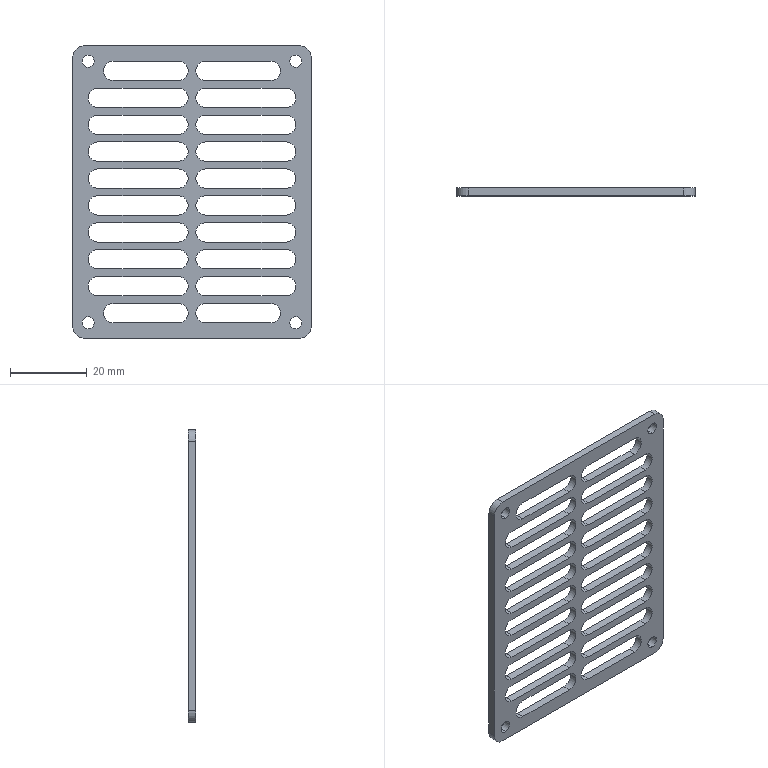Part | SolidWorks | features Extrusion 1, Fillet 1 | 1 solid | 98 faces | box 62 x 2 x 76 mm | volume 4523 mm3 | cylinder 52 | plane 46 | commonest cylinder face diameters 5 x40 3.1 x8 6 x4